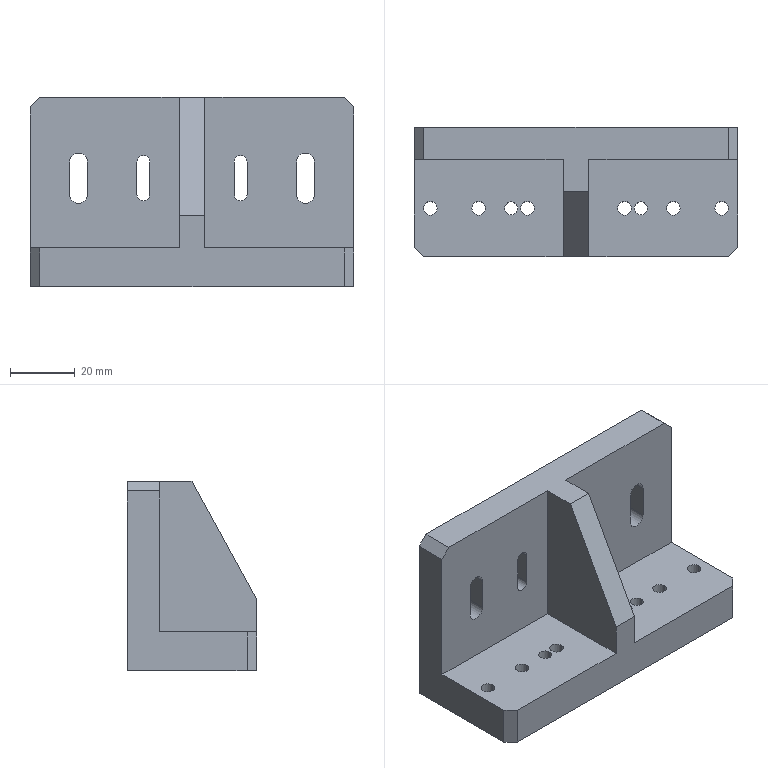Part | SolidWorks | features ICE 3, Chamfer 1, Extrusion 1, HoleWzd 1, Rib 1 | 1 solid | 49 faces | box 100 x 40 x 58.5 mm | volume 98616 mm3 | plane 25 | cylinder 24 | commonest cylinder face diameters 4.2 x12 4 x8 5.5 x4